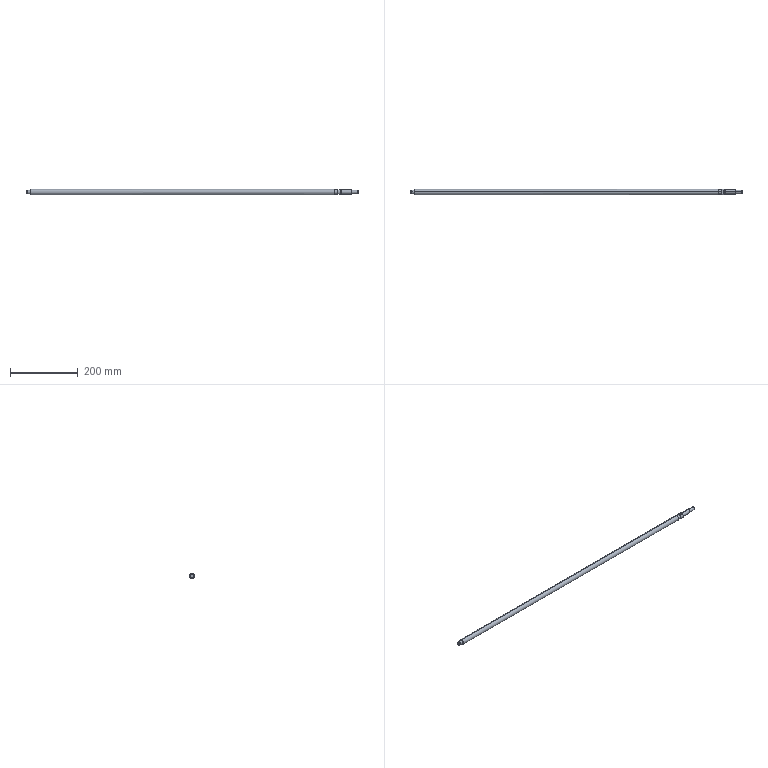Part | STEP file | Ball screw 4R16-16S2-DFSH-920-982-0.05(R)_HIWIN | 1 solid | 44 faces | box 982 x 16 x 16 mm | volume 189994 mm3 | cylinder 17 | plane 17 | cone 10 | commonest cylinder face diameters 10 x6 16 x4 9.6 x2 12 x2 13 x2 3 x1
STEP:
#1=CARTESIAN_POINT('',(-919.5,8.,0.));
#2=VERTEX_POINT('',#1);
#3=CARTESIAN_POINT('',(-919.5,0.,8.));
#4=VERTEX_POINT('',#3);
#5=CARTESIAN_POINT('',(-919.5,0.,0.));
#6=DIRECTION('',(1.,0.,0.));
#7=DIRECTION('',(0.,0.,-1.));
#8=AXIS2_PLACEMENT_3D('',#5,#6,#7);
#9=CIRCLE('',#8,8.);
#10=EDGE_CURVE('',#2,#4,#9,.T.);
#11=ORIENTED_EDGE('',*,*,#10,.T.);
#12=CARTESIAN_POINT('',(-20.,0.,8.));
#13=VERTEX_POINT('',#12);
#14=CARTESIAN_POINT('',(40.657,0.,8.));
#15=DIRECTION('',(1.,0.,0.));
#16=VECTOR('',#15,1000.);
#17=LINE('',#14,#16);
#18=EDGE_CURVE('',#4,#13,#17,.T.);
#19=ORIENTED_EDGE('',*,*,#18,.T.);
#20=CARTESIAN_POINT('',(-20.,0.,-8.));
#21=VERTEX_POINT('',#20);
#22=CARTESIAN_POINT('',(-20.,0.,0.));
#23=DIRECTION('',(-1.,0.,0.));
#24=DIRECTION('',(0.,0.,-1.));
#25=AXIS2_PLACEMENT_3D('',#22,#23,#24);
#26=CIRCLE('',#25,8.);
#27=EDGE_CURVE('',#13,#21,#26,.T.);
#28=ORIENTED_EDGE('',*,*,#27,.T.);
#29=CARTESIAN_POINT('',(-919.5,0.,-8.));
#30=VERTEX_POINT('',#29);
#31=CARTESIAN_POINT('',(40.657,0.,-8.));
#32=DIRECTION('',(1.,0.,0.));
#33=VECTOR('',#32,1000.);
#34=LINE('',#31,#33);
#35=EDGE_CURVE('',#30,#21,#34,.T.);
#36=ORIENTED_EDGE('',*,*,#35,.F.);
#37=CARTESIAN_POINT('',(-919.5,0.,0.));
#38=DIRECTION('',(1.,0.,0.));
#39=DIRECTION('',(0.,0.,-1.));
#40=AXIS2_PLACEMENT_3D('',#37,#38,#39);
#41=CIRCLE('',#40,8.);
#42=EDGE_CURVE('',#30,#2,#41,.T.);
#43=ORIENTED_EDGE('',*,*,#42,.T.);
#44=EDGE_LOOP('',(#11,#19,#28,#36,#43));
#45=FACE_OUTER_BOUND('',#44,.T.);
#46=CARTESIAN_POINT('',(40.657,0.,0.));
#47=DIRECTION('',(1.,0.,0.));
#48=DIRECTION('',(0.,0.,-1.));
#49=AXIS2_PLACEMENT_3D('',#46,#47,#48);
#50=CYLINDRICAL_SURFACE('',#49,8.);
#51=ADVANCED_FACE('',(#45),#50,.T.);
#52=CARTESIAN_POINT('',(-920.,7.5,0.));
#53=VERTEX_POINT('',#52);
#54=CARTESIAN_POINT('',(-920.,-7.5,0.));
#55=VERTEX_POINT('',#54);
#56=CARTESIAN_POINT('',(-920.,0.,0.));
#57=DIRECTION('',(1.,0.,0.));
#58=DIRECTION('',(0.,1.,0.));
#59=AXIS2_PLACEMENT_3D('',#56,#57,#58);
#60=CIRCLE('',#59,7.5);
#61=EDGE_CURVE('',#53,#55,#60,.T.);
#62=ORIENTED_EDGE('',*,*,#61,.T.);
#63=CARTESIAN_POINT('',(-919.5,-8.,0.));
#64=VERTEX_POINT('',#63);
#65=CARTESIAN_POINT('',(-919.5,-8.,0.));
#66=DIRECTION('',(0.7071,-0.7071,0.));
#67=VECTOR('',#66,1000.);
#68=LINE('',#65,#67);
#69=EDGE_CURVE('',#55,#64,#68,.T.);
#70=ORIENTED_EDGE('',*,*,#69,.T.);
#71=CARTESIAN_POINT('',(-919.5,0.,0.));
#72=DIRECTION('',(1.,0.,0.));
#73=DIRECTION('',(0.,0.,-1.));
#74=AXIS2_PLACEMENT_3D('',#71,#72,#73);
#75=CIRCLE('',#74,8.);
#76=EDGE_CURVE('',#4,#64,#75,.T.);
#77=ORIENTED_EDGE('',*,*,#76,.F.);
#78=ORIENTED_EDGE('',*,*,#10,.F.);
#79=CARTESIAN_POINT('',(-919.5,8.,0.));
#80=DIRECTION('',(0.7071,0.7071,0.));
#81=VECTOR('',#80,1000.);
#82=LINE('',#79,#81);
#83=EDGE_CURVE('',#53,#2,#82,.T.);
#84=ORIENTED_EDGE('',*,*,#83,.F.);
#85=EDGE_LOOP('',(#62,#70,#77,#78,#84));
#86=FACE_OUTER_BOUND('',#85,.T.);
#87=CARTESIAN_POINT('',(-919.5,0.,0.));
#88=DIRECTION('',(1.,0.,0.));
#89=DIRECTION('',(0.,1.,0.));
#90=AXIS2_PLACEMENT_3D('',#87,#88,#89);
#91=CONICAL_SURFACE('',#90,8.,0.7854);
#92=ADVANCED_FACE('',(#86),#91,.T.);
#93=CARTESIAN_POINT('',(-20.,0.,6.5));
#94=VERTEX_POINT('',#93);
#95=CARTESIAN_POINT('',(-20.,0.,-6.5));
#96=VERTEX_POINT('',#95);
#97=CARTESIAN_POINT('',(-20.,0.,0.));
#98=DIRECTION('',(-1.,0.,0.));
#99=DIRECTION('',(0.,0.,-1.));
#100=AXIS2_PLACEMENT_3D('',#97,#98,#99);
#101=CIRCLE('',#100,6.5);
#102=EDGE_CURVE('',#94,#96,#101,.T.);
#103=ORIENTED_EDGE('',*,*,#102,.F.);
#104=CARTESIAN_POINT('',(-10.,0.,6.5));
#105=VERTEX_POINT('',#104);
#106=CARTESIAN_POINT('',(-20.,0.,6.5));
#107=DIRECTION('',(1.,0.,0.));
#108=VECTOR('',#107,1000.);
#109=LINE('',#106,#108);
#110=EDGE_CURVE('',#94,#105,#109,.T.);
#111=ORIENTED_EDGE('',*,*,#110,.T.);
#112=CARTESIAN_POINT('',(-10.,0.,-6.5));
#113=VERTEX_POINT('',#112);
#114=CARTESIAN_POINT('',(-10.,0.,0.));
#115=DIRECTION('',(-1.,0.,0.));
#116=DIRECTION('',(0.,0.,-1.));
#117=AXIS2_PLACEMENT_3D('',#114,#115,#116);
#118=CIRCLE('',#117,6.5);
#119=EDGE_CURVE('',#105,#113,#118,.T.);
#120=ORIENTED_EDGE('',*,*,#119,.T.);
#121=CARTESIAN_POINT('',(-20.,0.,-6.5));
#122=DIRECTION('',(1.,0.,0.));
#123=VECTOR('',#122,1000.);
#124=LINE('',#121,#123);
#125=EDGE_CURVE('',#96,#113,#124,.T.);
#126=ORIENTED_EDGE('',*,*,#125,.F.);
#127=EDGE_LOOP('',(#103,#111,#120,#126));
#128=FACE_OUTER_BOUND('',#127,.T.);
#129=CARTESIAN_POINT('',(-20.,0.,0.));
#130=DIRECTION('',(1.,0.,0.));
#131=DIRECTION('',(0.,0.,-1.));
#132=AXIS2_PLACEMENT_3D('',#129,#130,#131);
#133=CYLINDRICAL_SURFACE('',#132,6.5);
#134=ADVANCED_FACE('',(#128),#133,.T.);
#135=CARTESIAN_POINT('',(-928.,0.,-5.));
#136=VERTEX_POINT('',#135);
#137=CARTESIAN_POINT('',(-928.,0.,5.));
#138=VERTEX_POINT('',#137);
#139=CARTESIAN_POINT('',(-928.,0.,0.));
#140=DIRECTION('',(1.,0.,0.));
#141=DIRECTION('',(0.,0.,-1.));
#142=AXIS2_PLACEMENT_3D('',#139,#140,#141);
#143=CIRCLE('',#142,5.);
#144=EDGE_CURVE('',#136,#138,#143,.T.);
#145=ORIENTED_EDGE('',*,*,#144,.T.);
#146=CARTESIAN_POINT('',(-920.,0.,5.));
#147=VERTEX_POINT('',#146);
#148=CARTESIAN_POINT('',(40.657,0.,5.));
#149=DIRECTION('',(1.,0.,0.));
#150=VECTOR('',#149,1000.);
#151=LINE('',#148,#150);
#152=EDGE_CURVE('',#138,#147,#151,.T.);
#153=ORIENTED_EDGE('',*,*,#152,.T.);
#154=CARTESIAN_POINT('',(-920.,0.,-5.));
#155=VERTEX_POINT('',#154);
#156=CARTESIAN_POINT('',(-920.,0.,0.));
#157=DIRECTION('',(1.,0.,0.));
#158=DIRECTION('',(0.,0.,-1.));
#159=AXIS2_PLACEMENT_3D('',#156,#157,#158);
#160=CIRCLE('',#159,5.);
#161=EDGE_CURVE('',#155,#147,#160,.T.);
#162=ORIENTED_EDGE('',*,*,#161,.F.);
#163=CARTESIAN_POINT('',(40.657,0.,-5.));
#164=DIRECTION('',(1.,0.,0.));
#165=VECTOR('',#164,1000.);
#166=LINE('',#163,#165);
#167=EDGE_CURVE('',#136,#155,#166,.T.);
#168=ORIENTED_EDGE('',*,*,#167,.F.);
#169=EDGE_LOOP('',(#145,#153,#162,#168));
#170=FACE_OUTER_BOUND('',#169,.T.);
#171=CARTESIAN_POINT('',(40.657,0.,0.));
#172=DIRECTION('',(1.,0.,0.));
#173=DIRECTION('',(0.,0.,-1.));
#174=AXIS2_PLACEMENT_3D('',#171,#172,#173);
#175=CYLINDRICAL_SURFACE('',#174,5.);
#176=ADVANCED_FACE('',(#170),#175,.T.);
#177=CARTESIAN_POINT('',(-5.,4.664,6.5));
#178=VERTEX_POINT('',#177);
#179=CARTESIAN_POINT('',(-5.,0.,8.));
#180=VERTEX_POINT('',#179);
#181=CARTESIAN_POINT('',(-5.,0.,0.));
#182=DIRECTION('',(1.,0.,0.));
#183=DIRECTION('',(0.,0.,-1.));
#184=AXIS2_PLACEMENT_3D('',#181,#182,#183);
#185=CIRCLE('',#184,8.);
#186=EDGE_CURVE('',#178,#180,#185,.T.);
#187=ORIENTED_EDGE('',*,*,#186,.T.);
#188=CARTESIAN_POINT('',(-0.5,0.,8.));
#189=VERTEX_POINT('',#188);
#190=CARTESIAN_POINT('',(40.657,0.,8.));
#191=DIRECTION('',(1.,0.,0.));
#192=VECTOR('',#191,1000.);
#193=LINE('',#190,#192);
#194=EDGE_CURVE('',#180,#189,#193,.T.);
#195=ORIENTED_EDGE('',*,*,#194,.T.);
#196=CARTESIAN_POINT('',(-0.5,0.,-8.));
#197=VERTEX_POINT('',#196);
#198=CARTESIAN_POINT('',(-0.5,0.,0.));
#199=DIRECTION('',(-1.,0.,0.));
#200=DIRECTION('',(0.,0.,-1.));
#201=AXIS2_PLACEMENT_3D('',#198,#199,#200);
#202=CIRCLE('',#201,8.);
#203=EDGE_CURVE('',#189,#197,#202,.T.);
#204=ORIENTED_EDGE('',*,*,#203,.T.);
#205=CARTESIAN_POINT('',(-5.,0.,-8.));
#206=VERTEX_POINT('',#205);
#207=CARTESIAN_POINT('',(40.657,0.,-8.));
#208=DIRECTION('',(1.,0.,0.));
#209=VECTOR('',#208,1000.);
#210=LINE('',#207,#209);
#211=EDGE_CURVE('',#206,#197,#210,.T.);
#212=ORIENTED_EDGE('',*,*,#211,.F.);
#213=CARTESIAN_POINT('',(-5.,4.664,-6.5));
#214=VERTEX_POINT('',#213);
#215=CARTESIAN_POINT('',(-5.,0.,0.));
#216=DIRECTION('',(1.,0.,0.));
#217=DIRECTION('',(0.,0.,-1.));
#218=AXIS2_PLACEMENT_3D('',#215,#216,#217);
#219=CIRCLE('',#218,8.);
#220=EDGE_CURVE('',#206,#214,#219,.T.);
#221=ORIENTED_EDGE('',*,*,#220,.T.);
#222=CARTESIAN_POINT('',(-10.,4.664,-6.5));
#223=VERTEX_POINT('',#222);
#224=CARTESIAN_POINT('',(-10.,4.664,-6.5));
#225=DIRECTION('',(-1.,0.,0.));
#226=VECTOR('',#225,1000.);
#227=LINE('',#224,#226);
#228=EDGE_CURVE('',#214,#223,#227,.T.);
#229=ORIENTED_EDGE('',*,*,#228,.T.);
#230=CARTESIAN_POINT('',(-10.,4.664,6.5));
#231=VERTEX_POINT('',#230);
#232=CARTESIAN_POINT('',(-10.,0.,0.));
#233=DIRECTION('',(1.,0.,0.));
#234=DIRECTION('',(0.,0.,-1.));
#235=AXIS2_PLACEMENT_3D('',#232,#233,#234);
#236=CIRCLE('',#235,8.);
#237=EDGE_CURVE('',#223,#231,#236,.T.);
#238=ORIENTED_EDGE('',*,*,#237,.T.);
#239=CARTESIAN_POINT('',(-10.,4.664,6.5));
#240=DIRECTION('',(1.,0.,0.));
#241=VECTOR('',#240,1000.);
#242=LINE('',#239,#241);
#243=EDGE_CURVE('',#231,#178,#242,.T.);
#244=ORIENTED_EDGE('',*,*,#243,.T.);
#245=EDGE_LOOP('',(#187,#195,#204,#212,#221,#229,#238,#244));
#246=FACE_OUTER_BOUND('',#245,.T.);
#247=CARTESIAN_POINT('',(40.657,0.,0.));
#248=DIRECTION('',(1.,0.,0.));
#249=DIRECTION('',(0.,0.,-1.));
#250=AXIS2_PLACEMENT_3D('',#247,#248,#249);
#251=CYLINDRICAL_SURFACE('',#250,8.);
#252=ADVANCED_FACE('',(#246),#251,.T.);
#253=CARTESIAN_POINT('',(0.,0.,7.5));
#254=VERTEX_POINT('',#253);
#255=CARTESIAN_POINT('',(0.,0.,-7.5));
#256=VERTEX_POINT('',#255);
#257=CARTESIAN_POINT('',(0.,0.,0.));
#258=DIRECTION('',(-1.,0.,0.));
#259=DIRECTION('',(0.,0.,1.));
#260=AXIS2_PLACEMENT_3D('',#257,#258,#259);
#261=CIRCLE('',#260,7.5);
#262=EDGE_CURVE('',#254,#256,#261,.T.);
#263=ORIENTED_EDGE('',*,*,#262,.T.);
#264=CARTESIAN_POINT('',(-0.5,0.,-8.));
#265=DIRECTION('',(-0.7071,0.,-0.7071));
#266=VECTOR('',#265,1000.);
#267=LINE('',#264,#266);
#268=EDGE_CURVE('',#256,#197,#267,.T.);
#269=ORIENTED_EDGE('',*,*,#268,.T.);
#270=ORIENTED_EDGE('',*,*,#203,.F.);
#271=CARTESIAN_POINT('',(-0.5,0.,8.));
#272=DIRECTION('',(-0.7071,0.,0.7071));
#273=VECTOR('',#272,1000.);
#274=LINE('',#271,#273);
#275=EDGE_CURVE('',#254,#189,#274,.T.);
#276=ORIENTED_EDGE('',*,*,#275,.F.);
#277=EDGE_LOOP('',(#263,#269,#270,#276));
#278=FACE_OUTER_BOUND('',#277,.T.);
#279=CARTESIAN_POINT('',(-0.5,0.,0.));
#280=DIRECTION('',(-1.,0.,0.));
#281=DIRECTION('',(0.,0.,1.));
#282=AXIS2_PLACEMENT_3D('',#279,#280,#281);
#283=CONICAL_SURFACE('',#282,8.,0.7854);
#284=ADVANCED_FACE('',(#278),#283,.T.);
#285=CARTESIAN_POINT('',(-929.15,0.,-4.8));
#286=VERTEX_POINT('',#285);
#287=CARTESIAN_POINT('',(-929.15,0.,4.8));
#288=VERTEX_POINT('',#287);
#289=CARTESIAN_POINT('',(-929.15,0.,0.));
#290=DIRECTION('',(1.,0.,0.));
#291=DIRECTION('',(0.,0.,-1.));
#292=AXIS2_PLACEMENT_3D('',#289,#290,#291);
#293=CIRCLE('',#292,4.8);
#294=EDGE_CURVE('',#286,#288,#293,.T.);
#295=ORIENTED_EDGE('',*,*,#294,.T.);
#296=CARTESIAN_POINT('',(-928.,0.,4.8));
#297=VERTEX_POINT('',#296);
#298=CARTESIAN_POINT('',(40.657,0.,4.8));
#299=DIRECTION('',(1.,0.,0.));
#300=VECTOR('',#299,1000.);
#301=LINE('',#298,#300);
#302=EDGE_CURVE('',#288,#297,#301,.T.);
#303=ORIENTED_EDGE('',*,*,#302,.T.);
#304=CARTESIAN_POINT('',(-928.,0.,-4.8));
#305=VERTEX_POINT('',#304);
#306=CARTESIAN_POINT('',(-928.,0.,0.));
#307=DIRECTION('',(1.,0.,0.));
#308=DIRECTION('',(0.,0.,-1.));
#309=AXIS2_PLACEMENT_3D('',#306,#307,#308);
#310=CIRCLE('',#309,4.8);
#311=EDGE_CURVE('',#305,#297,#310,.T.);
#312=ORIENTED_EDGE('',*,*,#311,.F.);
#313=CARTESIAN_POINT('',(40.657,0.,-4.8));
#314=DIRECTION('',(1.,0.,0.));
#315=VECTOR('',#314,1000.);
#316=LINE('',#313,#315);
#317=EDGE_CURVE('',#286,#305,#316,.T.);
#318=ORIENTED_EDGE('',*,*,#317,.F.);
#319=EDGE_LOOP('',(#295,#303,#312,#318));
#320=FACE_OUTER_BOUND('',#319,.T.);
#321=CARTESIAN_POINT('',(40.657,0.,0.));
#322=DIRECTION('',(1.,0.,0.));
#323=DIRECTION('',(0.,0.,-1.));
#324=AXIS2_PLACEMENT_3D('',#321,#322,#323);
#325=CYLINDRICAL_SURFACE('',#324,4.8);
#326=ADVANCED_FACE('',(#320),#325,.T.);
#327=CARTESIAN_POINT('',(0.,0.,6.));
#328=VERTEX_POINT('',#327);
#329=CARTESIAN_POINT('',(0.,0.,-6.));
#330=VERTEX_POINT('',#329);
#331=CARTESIAN_POINT('',(0.,0.,0.));
#332=DIRECTION('',(-1.,0.,0.));
#333=DIRECTION('',(0.,0.,-1.));
#334=AXIS2_PLACEMENT_3D('',#331,#332,#333);
#335=CIRCLE('',#334,6.);
#336=EDGE_CURVE('',#328,#330,#335,.T.);
#337=ORIENTED_EDGE('',*,*,#336,.F.);
#338=CARTESIAN_POINT('',(29.625,0.,6.));
#339=VERTEX_POINT('',#338);
#340=CARTESIAN_POINT('',(40.657,0.,6.));
#341=DIRECTION('',(1.,0.,0.));
#342=VECTOR('',#341,1000.);
#343=LINE('',#340,#342);
#344=EDGE_CURVE('',#328,#339,#343,.T.);
#345=ORIENTED_EDGE('',*,*,#344,.T.);
#346=CARTESIAN_POINT('',(29.625,0.,-6.));
#347=VERTEX_POINT('',#346);
#348=CARTESIAN_POINT('',(29.625,0.,0.));
#349=DIRECTION('',(-1.,0.,0.));
#350=DIRECTION('',(0.,0.,-1.));
#351=AXIS2_PLACEMENT_3D('',#348,#349,#350);
#352=CIRCLE('',#351,6.);
#353=EDGE_CURVE('',#339,#347,#352,.T.);
#354=ORIENTED_EDGE('',*,*,#353,.T.);
#355=CARTESIAN_POINT('',(40.657,0.,-6.));
#356=DIRECTION('',(1.,0.,0.));
#357=VECTOR('',#356,1000.);
#358=LINE('',#355,#357);
#359=EDGE_CURVE('',#330,#347,#358,.T.);
#360=ORIENTED_EDGE('',*,*,#359,.F.);
#361=EDGE_LOOP('',(#337,#345,#354,#360));
#362=FACE_OUTER_BOUND('',#361,.T.);
#363=CARTESIAN_POINT('',(40.657,0.,0.));
#364=DIRECTION('',(1.,0.,0.));
#365=DIRECTION('',(0.,0.,-1.));
#366=AXIS2_PLACEMENT_3D('',#363,#364,#365);
#367=CYLINDRICAL_SURFACE('',#366,6.);
#368=ADVANCED_FACE('',(#362),#367,.T.);
#369=CARTESIAN_POINT('',(-931.5,0.,-5.));
#370=VERTEX_POINT('',#369);
#371=CARTESIAN_POINT('',(-931.5,0.,5.));
#372=VERTEX_POINT('',#371);
#373=CARTESIAN_POINT('',(-931.5,0.,0.));
#374=DIRECTION('',(1.,0.,0.));
#375=DIRECTION('',(0.,0.,-1.));
#376=AXIS2_PLACEMENT_3D('',#373,#374,#375);
#377=CIRCLE('',#376,5.);
#378=EDGE_CURVE('',#370,#372,#377,.T.);
#379=ORIENTED_EDGE('',*,*,#378,.T.);
#380=CARTESIAN_POINT('',(-929.15,0.,5.));
#381=VERTEX_POINT('',#380);
#382=CARTESIAN_POINT('',(40.657,0.,5.));
#383=DIRECTION('',(1.,0.,0.));
#384=VECTOR('',#383,1000.);
#385=LINE('',#382,#384);
#386=EDGE_CURVE('',#372,#381,#385,.T.);
#387=ORIENTED_EDGE('',*,*,#386,.T.);
#388=CARTESIAN_POINT('',(-929.15,0.,-5.));
#389=VERTEX_POINT('',#388);
#390=CARTESIAN_POINT('',(-929.15,0.,0.));
#391=DIRECTION('',(1.,0.,0.));
#392=DIRECTION('',(0.,0.,-1.));
#393=AXIS2_PLACEMENT_3D('',#390,#391,#392);
#394=CIRCLE('',#393,5.);
#395=EDGE_CURVE('',#389,#381,#394,.T.);
#396=ORIENTED_EDGE('',*,*,#395,.F.);
#397=CARTESIAN_POINT('',(40.657,0.,-5.));
#398=DIRECTION('',(1.,0.,0.));
#399=VECTOR('',#398,1000.);
#400=LINE('',#397,#399);
#401=EDGE_CURVE('',#370,#389,#400,.T.);
#402=ORIENTED_EDGE('',*,*,#401,.F.);
#403=EDGE_LOOP('',(#379,#387,#396,#402));
#404=FACE_OUTER_BOUND('',#403,.T.);
#405=CARTESIAN_POINT('',(40.657,0.,0.));
#406=DIRECTION('',(1.,0.,0.));
#407=DIRECTION('',(0.,0.,-1.));
#408=AXIS2_PLACEMENT_3D('',#405,#406,#407);
#409=CYLINDRICAL_SURFACE('',#408,5.);
#410=ADVANCED_FACE('',(#404),#409,.T.);
#411=CARTESIAN_POINT('',(30.,0.,5.625));
#412=VERTEX_POINT('',#411);
#413=CARTESIAN_POINT('',(30.,0.,-5.625));
#414=VERTEX_POINT('',#413);
#415=CARTESIAN_POINT('',(30.,0.,0.));
#416=DIRECTION('',(-1.,0.,0.));
#417=DIRECTION('',(0.,0.,1.));
#418=AXIS2_PLACEMENT_3D('',#415,#416,#417);
#419=CIRCLE('',#418,5.625);
#420=EDGE_CURVE('',#412,#414,#419,.T.);
#421=ORIENTED_EDGE('',*,*,#420,.T.);
#422=CARTESIAN_POINT('',(29.625,0.,-6.));
#423=DIRECTION('',(-0.7071,0.,-0.7071));
#424=VECTOR('',#423,1000.);
#425=LINE('',#422,#424);
#426=EDGE_CURVE('',#414,#347,#425,.T.);
#427=ORIENTED_EDGE('',*,*,#426,.T.);
#428=ORIENTED_EDGE('',*,*,#353,.F.);
#429=CARTESIAN_POINT('',(29.625,0.,6.));
#430=DIRECTION('',(-0.7071,0.,0.7071));
#431=VECTOR('',#430,1000.);
#432=LINE('',#429,#431);
#433=EDGE_CURVE('',#412,#339,#432,.T.);
#434=ORIENTED_EDGE('',*,*,#433,.F.);
#435=EDGE_LOOP('',(#421,#427,#428,#434));
#436=FACE_OUTER_BOUND('',#435,.T.);
#437=CARTESIAN_POINT('',(29.625,0.,0.));
#438=DIRECTION('',(-1.,0.,0.));
#439=DIRECTION('',(0.,0.,1.));
#440=AXIS2_PLACEMENT_3D('',#437,#438,#439);
#441=CONICAL_SURFACE('',#440,6.,0.7854);
#442=ADVANCED_FACE('',(#436),#441,.T.);
#443=CARTESIAN_POINT('',(-932.,0.,-4.5));
#444=VERTEX_POINT('',#443);
#445=CARTESIAN_POINT('',(-932.,0.,4.5));
#446=VERTEX_POINT('',#445);
#447=CARTESIAN_POINT('',(-932.,0.,0.));
#448=DIRECTION('',(1.,0.,0.));
#449=DIRECTION('',(0.,0.,-1.));
#450=AXIS2_PLACEMENT_3D('',#447,#448,#449);
#451=CIRCLE('',#450,4.5);
#452=EDGE_CURVE('',#444,#446,#451,.T.);
#453=ORIENTED_EDGE('',*,*,#452,.T.);
#454=CARTESIAN_POINT('',(-931.5,0.,5.));
#455=DIRECTION('',(0.7071,0.,0.7071));
#456=VECTOR('',#455,1000.);
#457=LINE('',#454,#456);
#458=EDGE_CURVE('',#446,#372,#457,.T.);
#459=ORIENTED_EDGE('',*,*,#458,.T.);
#460=ORIENTED_EDGE('',*,*,#378,.F.);
#461=CARTESIAN_POINT('',(-931.5,0.,-5.));
#462=DIRECTION('',(0.7071,0.,-0.7071));
#463=VECTOR('',#462,1000.);
#464=LINE('',#461,#463);
#465=EDGE_CURVE('',#444,#370,#464,.T.);
#466=ORIENTED_EDGE('',*,*,#465,.F.);
#467=EDGE_LOOP('',(#453,#459,#460,#466));
#468=FACE_OUTER_BOUND('',#467,.T.);
#469=CARTESIAN_POINT('',(-931.5,0.,0.));
#470=DIRECTION('',(1.,0.,0.));
#471=DIRECTION('',(0.,0.,-1.));
#472=AXIS2_PLACEMENT_3D('',#469,#470,#471);
#473=CONICAL_SURFACE('',#472,5.,0.7854);
#474=ADVANCED_FACE('',(#468),#473,.T.);
#475=CARTESIAN_POINT('',(30.,0.,5.));
#476=VERTEX_POINT('',#475);
#477=CARTESIAN_POINT('',(30.,0.,-5.));
#478=VERTEX_POINT('',#477);
#479=CARTESIAN_POINT('',(30.,0.,0.));
#480=DIRECTION('',(-1.,0.,0.));
#481=DIRECTION('',(0.,0.,-1.));
#482=AXIS2_PLACEMENT_3D('',#479,#480,#481);
#483=CIRCLE('',#482,5.);
#484=EDGE_CURVE('',#476,#478,#483,.T.);
#485=ORIENTED_EDGE('',*,*,#484,.F.);
#486=CARTESIAN_POINT('',(49.5,0.,5.));
#487=VERTEX_POINT('',#486);
#488=CARTESIAN_POINT('',(40.657,0.,5.));
#489=DIRECTION('',(1.,0.,0.));
#490=VECTOR('',#489,1000.);
#491=LINE('',#488,#490);
#492=EDGE_CURVE('',#476,#487,#491,.T.);
#493=ORIENTED_EDGE('',*,*,#492,.T.);
#494=CARTESIAN_POINT('',(49.5,4.77,1.5));
#495=VERTEX_POINT('',#494);
#496=CARTESIAN_POINT('',(49.5,0.,0.));
#497=DIRECTION('',(-1.,0.,0.));
#498=DIRECTION('',(0.,0.,-1.));
#499=AXIS2_PLACEMENT_3D('',#496,#497,#498);
#500=CIRCLE('',#499,5.);
#501=EDGE_CURVE('',#487,#495,#500,.T.);
#502=ORIENTED_EDGE('',*,*,#501,.T.);
#503=CARTESIAN_POINT('',(35.5,4.77,1.5));
#504=VERTEX_POINT('',#503);
#505=CARTESIAN_POINT('',(40.657,4.77,1.5));
#506=DIRECTION('',(-1.,0.,0.));
#507=VECTOR('',#506,1000.);
#508=LINE('',#505,#507);
#509=EDGE_CURVE('',#495,#504,#508,.T.);
#510=ORIENTED_EDGE('',*,*,#509,.T.);
#511=CARTESIAN_POINT('',(35.5,4.77,-1.5));
#512=VERTEX_POINT('',#511);
#513=CARTESIAN_POINT('',(35.5,4.77,1.5));
#514=CARTESIAN_POINT('',(35.4,4.77,1.5));
#515=CARTESIAN_POINT('',(35.302,4.773,1.49));
#516=CARTESIAN_POINT('',(35.11,4.785,1.452));
#517=CARTESIAN_POINT('',(35.014,4.794,1.423));
#518=CARTESIAN_POINT('',(34.833,4.815,1.347));
#519=CARTESIAN_POINT('',(34.747,4.828,1.301));
#520=CARTESIAN_POINT('',(34.585,4.856,1.192));
#521=CARTESIAN_POINT('',(34.508,4.871,1.129));
#522=CARTESIAN_POINT('',(34.302,4.916,0.9233));
#523=CARTESIAN_POINT('',(34.19,4.946,0.7569));
#524=CARTESIAN_POINT('',(34.04,4.988,0.3965));
#525=CARTESIAN_POINT('',(34.,5.,0.1984));
#526=CARTESIAN_POINT('',(34.,5.,-0.09698));
#527=CARTESIAN_POINT('',(34.01,4.997,-0.197));
#528=CARTESIAN_POINT('',(34.048,4.986,-0.3898));
#529=CARTESIAN_POINT('',(34.077,4.977,-0.4837));
#530=CARTESIAN_POINT('',(34.19,4.946,-0.7572));
#531=CARTESIAN_POINT('',(34.301,4.916,-0.9219));
#532=CARTESIAN_POINT('',(34.508,4.871,-1.13));
#533=CARTESIAN_POINT('',(34.583,4.856,-1.191));
#534=CARTESIAN_POINT('',(34.745,4.828,-1.3));
#535=CARTESIAN_POINT('',(34.833,4.815,-1.347));
#536=CARTESIAN_POINT('',(35.104,4.783,-1.46));
#537=CARTESIAN_POINT('',(35.301,4.77,-1.5));
#538=CARTESIAN_POINT('',(35.5,4.77,-1.5));
#539=B_SPLINE_CURVE_WITH_KNOTS('',3,(#513,#514,#515,#516,#517,#518,#519,#520,#521,#522,#523,#524,#525,#526,#527,#528,#529,#530,#531,#532,#533,#534,#535,#536,#537,#538),.UNSPECIFIED.,.F.,.F.,(4,2,2,2,2,2,2,2,2,2,2,2,4),(0.,0.0002947,0.0005894,0.0008841,0.001179,0.001768,0.002358,0.002652,0.002947,0.003536,0.003831,0.004126,0.004715),.UNSPECIFIED.);
#540=EDGE_CURVE('',#504,#512,#539,.T.);
#541=ORIENTED_EDGE('',*,*,#540,.T.);
#542=CARTESIAN_POINT('',(49.5,4.77,-1.5));
#543=VERTEX_POINT('',#542);
#544=CARTESIAN_POINT('',(40.657,4.77,-1.5));
#545=DIRECTION('',(1.,0.,0.));
#546=VECTOR('',#545,1000.);
#547=LINE('',#544,#546);
#548=EDGE_CURVE('',#512,#543,#547,.T.);
#549=ORIENTED_EDGE('',*,*,#548,.T.);
#550=CARTESIAN_POINT('',(49.5,0.,-5.));
#551=VERTEX_POINT('',#550);
#552=CARTESIAN_POINT('',(49.5,0.,0.));
#553=DIRECTION('',(-1.,0.,0.));
#554=DIRECTION('',(0.,0.,-1.));
#555=AXIS2_PLACEMENT_3D('',#552,#553,#554);
#556=CIRCLE('',#555,5.);
#557=EDGE_CURVE('',#543,#551,#556,.T.);
#558=ORIENTED_EDGE('',*,*,#557,.T.);
#559=CARTESIAN_POINT('',(40.657,0.,-5.));
#560=DIRECTION('',(1.,0.,0.));
#561=VECTOR('',#560,1000.);
#562=LINE('',#559,#561);
#563=EDGE_CURVE('',#478,#551,#562,.T.);
#564=ORIENTED_EDGE('',*,*,#563,.F.);
#565=EDGE_LOOP('',(#485,#493,#502,#510,#541,#549,#558,#564));
#566=FACE_OUTER_BOUND('',#565,.T.);
#567=CARTESIAN_POINT('',(40.657,0.,0.));
#568=DIRECTION('',(1.,0.,0.));
#569=DIRECTION('',(0.,0.,-1.));
#570=AXIS2_PLACEMENT_3D('',#567,#568,#569);
#571=CYLINDRICAL_SURFACE('',#570,5.);
#572=ADVANCED_FACE('',(#566),#571,.T.);
#573=CARTESIAN_POINT('',(50.,4.243,-1.5));
#574=VERTEX_POINT('',#573);
#575=CARTESIAN_POINT('',(50.,-4.5,0.));
#576=VERTEX_POINT('',#575);
#577=CARTESIAN_POINT('',(50.,0.,0.));
#578=DIRECTION('',(-1.,0.,0.));
#579=DIRECTION('',(0.,-1.,0.));
#580=AXIS2_PLACEMENT_3D('',#577,#578,#579);
#581=CIRCLE('',#580,4.5);
#582=EDGE_CURVE('',#574,#576,#581,.T.);
#583=ORIENTED_EDGE('',*,*,#582,.T.);
#584=CARTESIAN_POINT('',(49.5,-5.,0.));
#585=VERTEX_POINT('',#584);
#586=CARTESIAN_POINT('',(49.5,-5.,0.));
#587=DIRECTION('',(-0.7071,-0.7071,0.));
#588=VECTOR('',#587,1000.);
#589=LINE('',#586,#588);
#590=EDGE_CURVE('',#576,#585,#589,.T.);
#591=ORIENTED_EDGE('',*,*,#590,.T.);
#592=CARTESIAN_POINT('',(49.5,0.,0.));
#593=DIRECTION('',(-1.,0.,0.));
#594=DIRECTION('',(0.,0.,-1.));
#595=AXIS2_PLACEMENT_3D('',#592,#593,#594);
#596=CIRCLE('',#595,5.);
#597=EDGE_CURVE('',#551,#585,#596,.T.);
#598=ORIENTED_EDGE('',*,*,#597,.F.);
#599=ORIENTED_EDGE('',*,*,#557,.F.);
#600=CARTESIAN_POINT('',(49.5,4.77,-1.5));
#601=CARTESIAN_POINT('',(49.667,4.594,-1.5));
#602=CARTESIAN_POINT('',(49.834,4.419,-1.5));
#603=CARTESIAN_POINT('',(50.,4.243,-1.5));
#604=B_SPLINE_CURVE_WITH_KNOTS('',3,(#600,#601,#602,#603),.UNSPECIFIED.,.F.,.F.,(4,4),(0.,0.0007265),.UNSPECIFIED.);
#605=EDGE_CURVE('',#543,#574,#604,.T.);
#606=ORIENTED_EDGE('',*,*,#605,.T.);
#607=EDGE_LOOP('',(#583,#591,#598,#599,#606));
#608=FACE_OUTER_BOUND('',#607,.T.);
#609=CARTESIAN_POINT('',(49.5,0.,0.));
#610=DIRECTION('',(-1.,0.,0.));
#611=DIRECTION('',(0.,-1.,0.));
#612=AXIS2_PLACEMENT_3D('',#609,#610,#611);
#613=CONICAL_SURFACE('',#612,5.,0.7854);
#614=ADVANCED_FACE('',(#608),#613,.T.);
#615=ORIENTED_EDGE('',*,*,#18,.F.);
#616=ORIENTED_EDGE('',*,*,#76,.T.);
#617=CARTESIAN_POINT('',(-919.5,0.,0.));
#618=DIRECTION('',(1.,0.,0.));
#619=DIRECTION('',(0.,0.,-1.));
#620=AXIS2_PLACEMENT_3D('',#617,#618,#619);
#621=CIRCLE('',#620,8.);
#622=EDGE_CURVE('',#64,#30,#621,.T.);
#623=ORIENTED_EDGE('',*,*,#622,.T.);
#624=ORIENTED_EDGE('',*,*,#35,.T.);
#625=CARTESIAN_POINT('',(-20.,0.,0.));
#626=DIRECTION('',(-1.,0.,0.));
#627=DIRECTION('',(0.,0.,-1.));
#628=AXIS2_PLACEMENT_3D('',#625,#626,#627);
#629=CIRCLE('',#628,8.);
#630=EDGE_CURVE('',#21,#13,#629,.T.);
#631=ORIENTED_EDGE('',*,*,#630,.T.);
#632=EDGE_LOOP('',(#615,#616,#623,#624,#631));
#633=FACE_OUTER_BOUND('',#632,.T.);
#634=CARTESIAN_POINT('',(40.657,0.,0.));
#635=DIRECTION('',(1.,0.,0.));
#636=DIRECTION('',(0.,0.,-1.));
#637=AXIS2_PLACEMENT_3D('',#634,#635,#636);
#638=CYLINDRICAL_SURFACE('',#637,8.);
#639=ADVANCED_FACE('',(#633),#638,.T.);
#640=ORIENTED_EDGE('',*,*,#630,.F.);
#641=ORIENTED_EDGE('',*,*,#27,.F.);
#642=EDGE_LOOP('',(#640,#641));
#643=FACE_OUTER_BOUND('',#642,.T.);
#644=CARTESIAN_POINT('',(-20.,0.,0.));
#645=DIRECTION('',(-1.,0.,0.));
#646=DIRECTION('',(0.,0.,-1.));
#647=AXIS2_PLACEMENT_3D('',#644,#645,#646);
#648=CIRCLE('',#647,6.5);
#649=EDGE_CURVE('',#96,#94,#648,.T.);
#650=ORIENTED_EDGE('',*,*,#649,.T.);
#651=ORIENTED_EDGE('',*,*,#102,.T.);
#652=EDGE_LOOP('',(#650,#651));
#653=FACE_BOUND('',#652,.T.);
#654=CARTESIAN_POINT('',(-20.,0.,0.));
#655=DIRECTION('',(1.,0.,0.));
#656=DIRECTION('',(0.,0.,-1.));
#657=AXIS2_PLACEMENT_3D('',#654,#655,#656);
#658=PLANE('',#657);
#659=ADVANCED_FACE('',(#643,#653),#658,.T.);
#660=ORIENTED_EDGE('',*,*,#69,.F.);
#661=CARTESIAN_POINT('',(-920.,0.,0.));
#662=DIRECTION('',(1.,0.,0.));
#663=DIRECTION('',(0.,1.,0.));
#664=AXIS2_PLACEMENT_3D('',#661,#662,#663);
#665=CIRCLE('',#664,7.5);
#666=EDGE_CURVE('',#55,#53,#665,.T.);
#667=ORIENTED_EDGE('',*,*,#666,.T.);
#668=ORIENTED_EDGE('',*,*,#83,.T.);
#669=ORIENTED_EDGE('',*,*,#42,.F.);
#670=ORIENTED_EDGE('',*,*,#622,.F.);
#671=EDGE_LOOP('',(#660,#667,#668,#669,#670));
#672=FACE_OUTER_BOUND('',#671,.T.);
#673=CARTESIAN_POINT('',(-919.5,0.,0.));
#674=DIRECTION('',(1.,0.,0.));
#675=DIRECTION('',(0.,1.,0.));
#676=AXIS2_PLACEMENT_3D('',#673,#674,#675);
#677=CONICAL_SURFACE('',#676,8.,0.7854);
#678=ADVANCED_FACE('',(#672),#677,.T.);
#679=ORIENTED_EDGE('',*,*,#110,.F.);
#680=ORIENTED_EDGE('',*,*,#649,.F.);
#681=ORIENTED_EDGE('',*,*,#125,.T.);
#682=CARTESIAN_POINT('',(-10.,0.,0.));
#683=DIRECTION('',(-1.,0.,0.));
#684=DIRECTION('',(0.,0.,-1.));
#685=AXIS2_PLACEMENT_3D('',#682,#683,#684);
#686=CIRCLE('',#685,6.5);
#687=EDGE_CURVE('',#113,#105,#686,.T.);
#688=ORIENTED_EDGE('',*,*,#687,.T.);
#689=EDGE_LOOP('',(#679,#680,#681,#688));
#690=FACE_OUTER_BOUND('',#689,.T.);
#691=CARTESIAN_POINT('',(-20.,0.,0.));
#692=DIRECTION('',(1.,0.,0.));
#693=DIRECTION('',(0.,0.,-1.));
#694=AXIS2_PLACEMENT_3D('',#691,#692,#693);
#695=CYLINDRICAL_SURFACE('',#694,6.5);
#696=ADVANCED_FACE('',(#690),#695,.T.);
#697=ORIENTED_EDGE('',*,*,#161,.T.);
#698=CARTESIAN_POINT('',(-920.,0.,0.));
#699=DIRECTION('',(1.,0.,0.));
#700=DIRECTION('',(0.,0.,-1.));
#701=AXIS2_PLACEMENT_3D('',#698,#699,#700);
#702=CIRCLE('',#701,5.);
#703=EDGE_CURVE('',#147,#155,#702,.T.);
#704=ORIENTED_EDGE('',*,*,#703,.T.);
#705=EDGE_LOOP('',(#697,#704));
#706=FACE_BOUND('',#705,.T.);
#707=ORIENTED_EDGE('',*,*,#61,.F.);
#708=ORIENTED_EDGE('',*,*,#666,.F.);
#709=EDGE_LOOP('',(#707,#708));
#710=FACE_OUTER_BOUND('',#709,.T.);
#711=CARTESIAN_POINT('',(-920.,8.,0.));
#712=DIRECTION('',(-1.,0.,0.));
#713=DIRECTION('',(0.,0.,1.));
#714=AXIS2_PLACEMENT_3D('',#711,#712,#713);
#715=PLANE('',#714);
#716=ADVANCED_FACE('',(#706,#710),#715,.T.);
#717=CARTESIAN_POINT('',(-10.,-4.664,6.5));
#718=VERTEX_POINT('',#717);
#719=CARTESIAN_POINT('',(-10.,0.,6.5));
#720=DIRECTION('',(0.,-1.,0.));
#721=VECTOR('',#720,1000.);
#722=LINE('',#719,#721);
#723=EDGE_CURVE('',#105,#718,#722,.T.);
#724=ORIENTED_EDGE('',*,*,#723,.F.);
#725=ORIENTED_EDGE('',*,*,#687,.F.);
#726=CARTESIAN_POINT('',(-10.,-4.664,-6.5));
#727=VERTEX_POINT('',#726);
#728=CARTESIAN_POINT('',(-10.,0.,-6.5));
#729=DIRECTION('',(0.,1.,0.));
#730=VECTOR('',#729,1000.);
#731=LINE('',#728,#730);
#732=EDGE_CURVE('',#727,#113,#731,.T.);
#733=ORIENTED_EDGE('',*,*,#732,.F.);
#734=CARTESIAN_POINT('',(-10.,0.,0.));
#735=DIRECTION('',(1.,0.,0.));
#736=DIRECTION('',(0.,0.,-1.));
#737=AXIS2_PLACEMENT_3D('',#734,#735,#736);
#738=CIRCLE('',#737,8.);
#739=EDGE_CURVE('',#718,#727,#738,.T.);
#740=ORIENTED_EDGE('',*,*,#739,.F.);
#741=EDGE_LOOP('',(#724,#725,#733,#740));
#742=FACE_OUTER_BOUND('',#741,.T.);
#743=CARTESIAN_POINT('',(-10.,0.,0.));
#744=DIRECTION('',(1.,0.,0.));
#745=DIRECTION('',(0.,0.,-1.));
#746=AXIS2_PLACEMENT_3D('',#743,#744,#745);
#747=PLANE('',#746);
#748=ADVANCED_FACE('',(#742),#747,.F.);
#749=CARTESIAN_POINT('',(-10.,0.,6.5));
#750=DIRECTION('',(0.,-1.,0.));
#751=VECTOR('',#750,1000.);
#752=LINE('',#749,#751);
#753=EDGE_CURVE('',#231,#105,#752,.T.);
#754=ORIENTED_EDGE('',*,*,#753,.F.);
#755=ORIENTED_EDGE('',*,*,#237,.F.);
#756=CARTESIAN_POINT('',(-10.,0.,-6.5));
#757=DIRECTION('',(0.,1.,0.));
#758=VECTOR('',#757,1000.);
#759=LINE('',#756,#758);
#760=EDGE_CURVE('',#113,#223,#759,.T.);
#761=ORIENTED_EDGE('',*,*,#760,.F.);
#762=ORIENTED_EDGE('',*,*,#119,.F.);
#763=EDGE_LOOP('',(#754,#755,#761,#762));
#764=FACE_OUTER_BOUND('',#763,.T.);
#765=CARTESIAN_POINT('',(-10.,0.,0.));
#766=DIRECTION('',(1.,0.,0.));
#767=DIRECTION('',(0.,0.,-1.));
#768=AXIS2_PLACEMENT_3D('',#765,#766,#767);
#769=PLANE('',#768);
#770=ADVANCED_FACE('',(#764),#769,.F.);
#771=ORIENTED_EDGE('',*,*,#152,.F.);
#772=CARTESIAN_POINT('',(-928.,0.,0.));
#773=DIRECTION('',(1.,0.,0.));
#774=DIRECTION('',(0.,0.,-1.));
#775=AXIS2_PLACEMENT_3D('',#772,#773,#774);
#776=CIRCLE('',#775,5.);
#777=EDGE_CURVE('',#138,#136,#776,.T.);
#778=ORIENTED_EDGE('',*,*,#777,.T.);
#779=ORIENTED_EDGE('',*,*,#167,.T.);
#780=ORIENTED_EDGE('',*,*,#703,.F.);
#781=EDGE_LOOP('',(#771,#778,#779,#780));
#782=FACE_OUTER_BOUND('',#781,.T.);
#783=CARTESIAN_POINT('',(40.657,0.,0.));
#784=DIRECTION('',(1.,0.,0.));
#785=DIRECTION('',(0.,0.,-1.));
#786=AXIS2_PLACEMENT_3D('',#783,#784,#785);
#787=CYLINDRICAL_SURFACE('',#786,5.);
#788=ADVANCED_FACE('',(#782),#787,.T.);
#789=ORIENTED_EDGE('',*,*,#194,.F.);
#790=CARTESIAN_POINT('',(-5.,-4.664,6.5));
#791=VERTEX_POINT('',#790);
#792=CARTESIAN_POINT('',(-5.,0.,0.));
#793=DIRECTION('',(1.,0.,0.));
#794=DIRECTION('',(0.,0.,-1.));
#795=AXIS2_PLACEMENT_3D('',#792,#793,#794);
#796=CIRCLE('',#795,8.);
#797=EDGE_CURVE('',#180,#791,#796,.T.);
#798=ORIENTED_EDGE('',*,*,#797,.T.);
#799=CARTESIAN_POINT('',(40.657,-4.664,6.5));
#800=DIRECTION('',(-1.,0.,0.));
#801=VECTOR('',#800,1000.);
#802=LINE('',#799,#801);
#803=EDGE_CURVE('',#791,#718,#802,.T.);
#804=ORIENTED_EDGE('',*,*,#803,.T.);
#805=ORIENTED_EDGE('',*,*,#739,.T.);
#806=CARTESIAN_POINT('',(-5.,-4.664,-6.5));
#807=VERTEX_POINT('',#806);
#808=CARTESIAN_POINT('',(40.657,-4.664,-6.5));
#809=DIRECTION('',(1.,0.,0.));
#810=VECTOR('',#809,1000.);
#811=LINE('',#808,#810);
#812=EDGE_CURVE('',#727,#807,#811,.T.);
#813=ORIENTED_EDGE('',*,*,#812,.T.);
#814=CARTESIAN_POINT('',(-5.,0.,0.));
#815=DIRECTION('',(1.,0.,0.));
#816=DIRECTION('',(0.,0.,-1.));
#817=AXIS2_PLACEMENT_3D('',#814,#815,#816);
#818=CIRCLE('',#817,8.);
#819=EDGE_CURVE('',#807,#206,#818,.T.);
#820=ORIENTED_EDGE('',*,*,#819,.T.);
#821=ORIENTED_EDGE('',*,*,#211,.T.);
#822=CARTESIAN_POINT('',(-0.5,0.,0.));
#823=DIRECTION('',(-1.,0.,0.));
#824=DIRECTION('',(0.,0.,-1.));
#825=AXIS2_PLACEMENT_3D('',#822,#823,#824);
#826=CIRCLE('',#825,8.);
#827=EDGE_CURVE('',#197,#189,#826,.T.);
#828=ORIENTED_EDGE('',*,*,#827,.T.);
#829=EDGE_LOOP('',(#789,#798,#804,#805,#813,#820,#821,#828));
#830=FACE_OUTER_BOUND('',#829,.T.);
#831=CARTESIAN_POINT('',(40.657,0.,0.));
#832=DIRECTION('',(1.,0.,0.));
#833=DIRECTION('',(0.,0.,-1.));
#834=AXIS2_PLACEMENT_3D('',#831,#832,#833);
#835=CYLINDRICAL_SURFACE('',#834,8.);
#836=ADVANCED_FACE('',(#830),#835,.T.);
#837=ORIENTED_EDGE('',*,*,#753,.T.);
#838=ORIENTED_EDGE('',*,*,#723,.T.);
#839=ORIENTED_EDGE('',*,*,#803,.F.);
#840=CARTESIAN_POINT('',(-5.,-8.,6.5));
#841=DIRECTION('',(0.,-1.,0.));
#842=VECTOR('',#841,1000.);
#843=LINE('',#840,#842);
#844=EDGE_CURVE('',#178,#791,#843,.T.);
#845=ORIENTED_EDGE('',*,*,#844,.F.);
#846=ORIENTED_EDGE('',*,*,#243,.F.);
#847=EDGE_LOOP('',(#837,#838,#839,#845,#846));
#848=FACE_OUTER_BOUND('',#847,.T.);
#849=CARTESIAN_POINT('',(-10.,-8.,6.5));
#850=DIRECTION('',(0.,0.,-1.));
#851=DIRECTION('',(-1.,0.,0.));
#852=AXIS2_PLACEMENT_3D('',#849,#850,#851);
#853=PLANE('',#852);
#854=ADVANCED_FACE('',(#848),#853,.F.);
#855=ORIENTED_EDGE('',*,*,#732,.T.);
#856=ORIENTED_EDGE('',*,*,#760,.T.);
#857=ORIENTED_EDGE('',*,*,#228,.F.);
#858=CARTESIAN_POINT('',(-5.,-8.,-6.5));
#859=DIRECTION('',(0.,1.,0.));
#860=VECTOR('',#859,1000.);
#861=LINE('',#858,#860);
#862=EDGE_CURVE('',#807,#214,#861,.T.);
#863=ORIENTED_EDGE('',*,*,#862,.F.);
#864=ORIENTED_EDGE('',*,*,#812,.F.);
#865=EDGE_LOOP('',(#855,#856,#857,#863,#864));
#866=FACE_OUTER_BOUND('',#865,.T.);
#867=CARTESIAN_POINT('',(-10.,-8.,-6.5));
#868=DIRECTION('',(0.,0.,1.));
#869=DIRECTION('',(1.,0.,0.));
#870=AXIS2_PLACEMENT_3D('',#867,#868,#869);
#871=PLANE('',#870);
#872=ADVANCED_FACE('',(#866),#871,.F.);
#873=ORIENTED_EDGE('',*,*,#144,.F.);
#874=ORIENTED_EDGE('',*,*,#777,.F.);
#875=EDGE_LOOP('',(#873,#874));
#876=FACE_OUTER_BOUND('',#875,.T.);
#877=ORIENTED_EDGE('',*,*,#311,.T.);
#878=CARTESIAN_POINT('',(-928.,0.,0.));
#879=DIRECTION('',(1.,0.,0.));
#880=DIRECTION('',(0.,0.,-1.));
#881=AXIS2_PLACEMENT_3D('',#878,#879,#880);
#882=CIRCLE('',#881,4.8);
#883=EDGE_CURVE('',#297,#305,#882,.T.);
#884=ORIENTED_EDGE('',*,*,#883,.T.);
#885=EDGE_LOOP('',(#877,#884));
#886=FACE_BOUND('',#885,.T.);
#887=CARTESIAN_POINT('',(-928.,5.,0.));
#888=DIRECTION('',(-1.,0.,0.));
#889=DIRECTION('',(0.,0.,1.));
#890=AXIS2_PLACEMENT_3D('',#887,#888,#889);
#891=PLANE('',#890);
#892=ADVANCED_FACE('',(#876,#886),#891,.T.);
#893=ORIENTED_EDGE('',*,*,#268,.F.);
#894=CARTESIAN_POINT('',(0.,0.,0.));
#895=DIRECTION('',(-1.,0.,0.));
#896=DIRECTION('',(0.,0.,1.));
#897=AXIS2_PLACEMENT_3D('',#894,#895,#896);
#898=CIRCLE('',#897,7.5);
#899=EDGE_CURVE('',#256,#254,#898,.T.);
#900=ORIENTED_EDGE('',*,*,#899,.T.);
#901=ORIENTED_EDGE('',*,*,#275,.T.);
#902=ORIENTED_EDGE('',*,*,#827,.F.);
#903=EDGE_LOOP('',(#893,#900,#901,#902));
#904=FACE_OUTER_BOUND('',#903,.T.);
#905=CARTESIAN_POINT('',(-0.5,0.,0.));
#906=DIRECTION('',(-1.,0.,0.));
#907=DIRECTION('',(0.,0.,1.));
#908=AXIS2_PLACEMENT_3D('',#905,#906,#907);
#909=CONICAL_SURFACE('',#908,8.,0.7854);
#910=ADVANCED_FACE('',(#904),#909,.T.);
#911=ORIENTED_EDGE('',*,*,#819,.F.);
#912=ORIENTED_EDGE('',*,*,#862,.T.);
#913=ORIENTED_EDGE('',*,*,#220,.F.);
#914=EDGE_LOOP('',(#911,#912,#913));
#915=FACE_OUTER_BOUND('',#914,.T.);
#916=CARTESIAN_POINT('',(-5.,-8.,-8.));
#917=DIRECTION('',(1.,0.,0.));
#918=DIRECTION('',(0.,0.,-1.));
#919=AXIS2_PLACEMENT_3D('',#916,#917,#918);
#920=PLANE('',#919);
#921=ADVANCED_FACE('',(#915),#920,.F.);
#922=ORIENTED_EDGE('',*,*,#186,.F.);
#923=ORIENTED_EDGE('',*,*,#844,.T.);
#924=ORIENTED_EDGE('',*,*,#797,.F.);
#925=EDGE_LOOP('',(#922,#923,#924));
#926=FACE_OUTER_BOUND('',#925,.T.);
#927=CARTESIAN_POINT('',(-5.,-8.,8.));
#928=DIRECTION('',(1.,0.,0.));
#929=DIRECTION('',(0.,0.,-1.));
#930=AXIS2_PLACEMENT_3D('',#927,#928,#929);
#931=PLANE('',#930);
#932=ADVANCED_FACE('',(#926),#931,.F.);
#933=ORIENTED_EDGE('',*,*,#302,.F.);
#934=CARTESIAN_POINT('',(-929.15,0.,0.));
#935=DIRECTION('',(1.,0.,0.));
#936=DIRECTION('',(0.,0.,-1.));
#937=AXIS2_PLACEMENT_3D('',#934,#935,#936);
#938=CIRCLE('',#937,4.8);
#939=EDGE_CURVE('',#288,#286,#938,.T.);
#940=ORIENTED_EDGE('',*,*,#939,.T.);
#941=ORIENTED_EDGE('',*,*,#317,.T.);
#942=ORIENTED_EDGE('',*,*,#883,.F.);
#943=EDGE_LOOP('',(#933,#940,#941,#942));
#944=FACE_OUTER_BOUND('',#943,.T.);
#945=CARTESIAN_POINT('',(40.657,0.,0.));
#946=DIRECTION('',(1.,0.,0.));
#947=DIRECTION('',(0.,0.,-1.));
#948=AXIS2_PLACEMENT_3D('',#945,#946,#947);
#949=CYLINDRICAL_SURFACE('',#948,4.8);
#950=ADVANCED_FACE('',(#944),#949,.T.);
#951=CARTESIAN_POINT('',(0.,0.,0.));
#952=DIRECTION('',(-1.,0.,0.));
#953=DIRECTION('',(0.,0.,-1.));
#954=AXIS2_PLACEMENT_3D('',#951,#952,#953);
#955=CIRCLE('',#954,6.);
#956=EDGE_CURVE('',#330,#328,#955,.T.);
#957=ORIENTED_EDGE('',*,*,#956,.T.);
#958=ORIENTED_EDGE('',*,*,#336,.T.);
#959=EDGE_LOOP('',(#957,#958));
#960=FACE_BOUND('',#959,.T.);
#961=ORIENTED_EDGE('',*,*,#262,.F.);
#962=ORIENTED_EDGE('',*,*,#899,.F.);
#963=EDGE_LOOP('',(#961,#962));
#964=FACE_OUTER_BOUND('',#963,.T.);
#965=CARTESIAN_POINT('',(0.,6.,0.));
#966=DIRECTION('',(1.,0.,0.));
#967=DIRECTION('',(0.,0.,-1.));
#968=AXIS2_PLACEMENT_3D('',#965,#966,#967);
#969=PLANE('',#968);
#970=ADVANCED_FACE('',(#960,#964),#969,.T.);
#971=ORIENTED_EDGE('',*,*,#294,.F.);
#972=ORIENTED_EDGE('',*,*,#939,.F.);
#973=EDGE_LOOP('',(#971,#972));
#974=FACE_BOUND('',#973,.T.);
#975=ORIENTED_EDGE('',*,*,#395,.T.);
#976=CARTESIAN_POINT('',(-929.15,0.,0.));
#977=DIRECTION('',(1.,0.,0.));
#978=DIRECTION('',(0.,0.,-1.));
#979=AXIS2_PLACEMENT_3D('',#976,#977,#978);
#980=CIRCLE('',#979,5.);
#981=EDGE_CURVE('',#381,#389,#980,.T.);
#982=ORIENTED_EDGE('',*,*,#981,.T.);
#983=EDGE_LOOP('',(#975,#982));
#984=FACE_OUTER_BOUND('',#983,.T.);
#985=CARTESIAN_POINT('',(-929.15,4.8,0.));
#986=DIRECTION('',(1.,0.,0.));
#987=DIRECTION('',(0.,0.,-1.));
#988=AXIS2_PLACEMENT_3D('',#985,#986,#987);
#989=PLANE('',#988);
#990=ADVANCED_FACE('',(#974,#984),#989,.T.);
#991=ORIENTED_EDGE('',*,*,#344,.F.);
#992=ORIENTED_EDGE('',*,*,#956,.F.);
#993=ORIENTED_EDGE('',*,*,#359,.T.);
#994=CARTESIAN_POINT('',(29.625,0.,0.));
#995=DIRECTION('',(-1.,0.,0.));
#996=DIRECTION('',(0.,0.,-1.));
#997=AXIS2_PLACEMENT_3D('',#994,#995,#996);
#998=CIRCLE('',#997,6.);
#999=EDGE_CURVE('',#347,#339,#998,.T.);
#1000=ORIENTED_EDGE('',*,*,#999,.T.);
#1001=EDGE_LOOP('',(#991,#992,#993,#1000));
#1002=FACE_OUTER_BOUND('',#1001,.T.);
#1003=CARTESIAN_POINT('',(40.657,0.,0.));
#1004=DIRECTION('',(1.,0.,0.));
#1005=DIRECTION('',(0.,0.,-1.));
#1006=AXIS2_PLACEMENT_3D('',#1003,#1004,#1005);
#1007=CYLINDRICAL_SURFACE('',#1006,6.);
#1008=ADVANCED_FACE('',(#1002),#1007,.T.);
#1009=ORIENTED_EDGE('',*,*,#386,.F.);
#1010=CARTESIAN_POINT('',(-931.5,0.,0.));
#1011=DIRECTION('',(1.,0.,0.));
#1012=DIRECTION('',(0.,0.,-1.));
#1013=AXIS2_PLACEMENT_3D('',#1010,#1011,#1012);
#1014=CIRCLE('',#1013,5.);
#1015=EDGE_CURVE('',#372,#370,#1014,.T.);
#1016=ORIENTED_EDGE('',*,*,#1015,.T.);
#1017=ORIENTED_EDGE('',*,*,#401,.T.);
#1018=ORIENTED_EDGE('',*,*,#981,.F.);
#1019=EDGE_LOOP('',(#1009,#1016,#1017,#1018));
#1020=FACE_OUTER_BOUND('',#1019,.T.);
#1021=CARTESIAN_POINT('',(40.657,0.,0.));
#1022=DIRECTION('',(1.,0.,0.));
#1023=DIRECTION('',(0.,0.,-1.));
#1024=AXIS2_PLACEMENT_3D('',#1021,#1022,#1023);
#1025=CYLINDRICAL_SURFACE('',#1024,5.);
#1026=ADVANCED_FACE('',(#1020),#1025,.T.);
#1027=ORIENTED_EDGE('',*,*,#426,.F.);
#1028=CARTESIAN_POINT('',(30.,0.,0.));
#1029=DIRECTION('',(-1.,0.,0.));
#1030=DIRECTION('',(0.,0.,1.));
#1031=AXIS2_PLACEMENT_3D('',#1028,#1029,#1030);
#1032=CIRCLE('',#1031,5.625);
#1033=EDGE_CURVE('',#414,#412,#1032,.T.);
#1034=ORIENTED_EDGE('',*,*,#1033,.T.);
#1035=ORIENTED_EDGE('',*,*,#433,.T.);
#1036=ORIENTED_EDGE('',*,*,#999,.F.);
#1037=EDGE_LOOP('',(#1027,#1034,#1035,#1036));
#1038=FACE_OUTER_BOUND('',#1037,.T.);
#1039=CARTESIAN_POINT('',(29.625,0.,0.));
#1040=DIRECTION('',(-1.,0.,0.));
#1041=DIRECTION('',(0.,0.,1.));
#1042=AXIS2_PLACEMENT_3D('',#1039,#1040,#1041);
#1043=CONICAL_SURFACE('',#1042,6.,0.7854);
#1044=ADVANCED_FACE('',(#1038),#1043,.T.);
#1045=ORIENTED_EDGE('',*,*,#458,.F.);
#1046=CARTESIAN_POINT('',(-932.,0.,0.));
#1047=DIRECTION('',(1.,0.,0.));
#1048=DIRECTION('',(0.,0.,-1.));
#1049=AXIS2_PLACEMENT_3D('',#1046,#1047,#1048);
#1050=CIRCLE('',#1049,4.5);
#1051=EDGE_CURVE('',#446,#444,#1050,.T.);
#1052=ORIENTED_EDGE('',*,*,#1051,.T.);
#1053=ORIENTED_EDGE('',*,*,#465,.T.);
#1054=ORIENTED_EDGE('',*,*,#1015,.F.);
#1055=EDGE_LOOP('',(#1045,#1052,#1053,#1054));
#1056=FACE_OUTER_BOUND('',#1055,.T.);
#1057=CARTESIAN_POINT('',(-931.5,0.,0.));
#1058=DIRECTION('',(1.,0.,0.));
#1059=DIRECTION('',(0.,0.,-1.));
#1060=AXIS2_PLACEMENT_3D('',#1057,#1058,#1059);
#1061=CONICAL_SURFACE('',#1060,5.,0.7854);
#1062=ADVANCED_FACE('',(#1056),#1061,.T.);
#1063=CARTESIAN_POINT('',(30.,0.,0.));
#1064=DIRECTION('',(-1.,0.,0.));
#1065=DIRECTION('',(0.,0.,-1.));
#1066=AXIS2_PLACEMENT_3D('',#1063,#1064,#1065);
#1067=CIRCLE('',#1066,5.);
#1068=EDGE_CURVE('',#478,#476,#1067,.T.);
#1069=ORIENTED_EDGE('',*,*,#1068,.T.);
#1070=ORIENTED_EDGE('',*,*,#484,.T.);
#1071=EDGE_LOOP('',(#1069,#1070));
#1072=FACE_BOUND('',#1071,.T.);
#1073=ORIENTED_EDGE('',*,*,#420,.F.);
#1074=ORIENTED_EDGE('',*,*,#1033,.F.);
#1075=EDGE_LOOP('',(#1073,#1074));
#1076=FACE_OUTER_BOUND('',#1075,.T.);
#1077=CARTESIAN_POINT('',(30.,5.,0.));
#1078=DIRECTION('',(1.,0.,0.));
#1079=DIRECTION('',(0.,0.,-1.));
#1080=AXIS2_PLACEMENT_3D('',#1077,#1078,#1079);
#1081=PLANE('',#1080);
#1082=ADVANCED_FACE('',(#1072,#1076),#1081,.T.);
#1083=ORIENTED_EDGE('',*,*,#452,.F.);
#1084=ORIENTED_EDGE('',*,*,#1051,.F.);
#1085=EDGE_LOOP('',(#1083,#1084));
#1086=FACE_OUTER_BOUND('',#1085,.T.);
#1087=CARTESIAN_POINT('',(-932.,5.,0.));
#1088=DIRECTION('',(-1.,0.,0.));
#1089=DIRECTION('',(0.,0.,1.));
#1090=AXIS2_PLACEMENT_3D('',#1087,#1088,#1089);
#1091=PLANE('',#1090);
#1092=ADVANCED_FACE('',(#1086),#1091,.T.);
#1093=ORIENTED_EDGE('',*,*,#492,.F.);
#1094=ORIENTED_EDGE('',*,*,#1068,.F.);
#1095=ORIENTED_EDGE('',*,*,#563,.T.);
#1096=ORIENTED_EDGE('',*,*,#597,.T.);
#1097=CARTESIAN_POINT('',(49.5,0.,0.));
#1098=DIRECTION('',(-1.,0.,0.));
#1099=DIRECTION('',(0.,0.,-1.));
#1100=AXIS2_PLACEMENT_3D('',#1097,#1098,#1099);
#1101=CIRCLE('',#1100,5.);
#1102=EDGE_CURVE('',#585,#487,#1101,.T.);
#1103=ORIENTED_EDGE('',*,*,#1102,.T.);
#1104=EDGE_LOOP('',(#1093,#1094,#1095,#1096,#1103));
#1105=FACE_OUTER_BOUND('',#1104,.T.);
#1106=CARTESIAN_POINT('',(40.657,0.,0.));
#1107=DIRECTION('',(1.,0.,0.));
#1108=DIRECTION('',(0.,0.,-1.));
#1109=AXIS2_PLACEMENT_3D('',#1106,#1107,#1108);
#1110=CYLINDRICAL_SURFACE('',#1109,5.);
#1111=ADVANCED_FACE('',(#1105),#1110,.T.);
#1112=ORIENTED_EDGE('',*,*,#590,.F.);
#1113=CARTESIAN_POINT('',(50.,4.243,1.5));
#1114=VERTEX_POINT('',#1113);
#1115=CARTESIAN_POINT('',(50.,0.,0.));
#1116=DIRECTION('',(-1.,0.,0.));
#1117=DIRECTION('',(0.,-1.,0.));
#1118=AXIS2_PLACEMENT_3D('',#1115,#1116,#1117);
#1119=CIRCLE('',#1118,4.5);
#1120=EDGE_CURVE('',#576,#1114,#1119,.T.);
#1121=ORIENTED_EDGE('',*,*,#1120,.T.);
#1122=CARTESIAN_POINT('',(49.5,4.77,1.5));
#1123=CARTESIAN_POINT('',(49.667,4.594,1.5));
#1124=CARTESIAN_POINT('',(49.834,4.419,1.5));
#1125=CARTESIAN_POINT('',(50.,4.243,1.5));
#1126=B_SPLINE_CURVE_WITH_KNOTS('',3,(#1122,#1123,#1124,#1125),.UNSPECIFIED.,.F.,.F.,(4,4),(0.,0.0007265),.UNSPECIFIED.);
#1127=EDGE_CURVE('',#495,#1114,#1126,.T.);
#1128=ORIENTED_EDGE('',*,*,#1127,.F.);
#1129=ORIENTED_EDGE('',*,*,#501,.F.);
#1130=ORIENTED_EDGE('',*,*,#1102,.F.);
#1131=EDGE_LOOP('',(#1112,#1121,#1128,#1129,#1130));
#1132=FACE_OUTER_BOUND('',#1131,.T.);
#1133=CARTESIAN_POINT('',(49.5,0.,0.));
#1134=DIRECTION('',(-1.,0.,0.));
#1135=DIRECTION('',(0.,-1.,0.));
#1136=AXIS2_PLACEMENT_3D('',#1133,#1134,#1135);
#1137=CONICAL_SURFACE('',#1136,5.,0.7854);
#1138=ADVANCED_FACE('',(#1132),#1137,.T.);
#1139=ORIENTED_EDGE('',*,*,#605,.F.);
#1140=ORIENTED_EDGE('',*,*,#548,.F.);
#1141=CARTESIAN_POINT('',(35.5,3.2,-1.5));
#1142=VERTEX_POINT('',#1141);
#1143=CARTESIAN_POINT('',(35.5,13.2,-1.5));
#1144=DIRECTION('',(0.,-1.,0.));
#1145=VECTOR('',#1144,1000.);
#1146=LINE('',#1143,#1145);
#1147=EDGE_CURVE('',#512,#1142,#1146,.T.);
#1148=ORIENTED_EDGE('',*,*,#1147,.T.);
#1149=CARTESIAN_POINT('',(50.,3.2,-1.5));
#1150=VERTEX_POINT('',#1149);
#1151=CARTESIAN_POINT('',(50.,3.2,-1.5));
#1152=DIRECTION('',(1.,0.,0.));
#1153=VECTOR('',#1152,1000.);
#1154=LINE('',#1151,#1153);
#1155=EDGE_CURVE('',#1142,#1150,#1154,.T.);
#1156=ORIENTED_EDGE('',*,*,#1155,.T.);
#1157=CARTESIAN_POINT('',(50.,13.2,-1.5));
#1158=DIRECTION('',(0.,1.,0.));
#1159=VECTOR('',#1158,1000.);
#1160=LINE('',#1157,#1159);
#1161=EDGE_CURVE('',#1150,#574,#1160,.T.);
#1162=ORIENTED_EDGE('',*,*,#1161,.T.);
#1163=EDGE_LOOP('',(#1139,#1140,#1148,#1156,#1162));
#1164=FACE_OUTER_BOUND('',#1163,.T.);
#1165=CARTESIAN_POINT('',(50.,13.2,-1.5));
#1166=DIRECTION('',(0.,0.,1.));
#1167=DIRECTION('',(1.,0.,0.));
#1168=AXIS2_PLACEMENT_3D('',#1165,#1166,#1167);
#1169=PLANE('',#1168);
#1170=ADVANCED_FACE('',(#1164),#1169,.T.);
#1171=CARTESIAN_POINT('',(35.5,3.2,1.5));
#1172=VERTEX_POINT('',#1171);
#1173=CARTESIAN_POINT('',(35.5,3.2,0.));
#1174=DIRECTION('',(0.,1.,0.));
#1175=DIRECTION('',(0.,0.,-1.));
#1176=AXIS2_PLACEMENT_3D('',#1173,#1174,#1175);
#1177=CIRCLE('',#1176,1.5);
#1178=EDGE_CURVE('',#1142,#1172,#1177,.T.);
#1179=ORIENTED_EDGE('',*,*,#1178,.F.);
#1180=ORIENTED_EDGE('',*,*,#1147,.F.);
#1181=ORIENTED_EDGE('',*,*,#540,.F.);
#1182=CARTESIAN_POINT('',(35.5,13.2,1.5));
#1183=DIRECTION('',(0.,1.,0.));
#1184=VECTOR('',#1183,1000.);
#1185=LINE('',#1182,#1184);
#1186=EDGE_CURVE('',#1172,#504,#1185,.T.);
#1187=ORIENTED_EDGE('',*,*,#1186,.F.);
#1188=EDGE_LOOP('',(#1179,#1180,#1181,#1187));
#1189=FACE_OUTER_BOUND('',#1188,.T.);
#1190=CARTESIAN_POINT('',(35.5,13.2,0.));
#1191=DIRECTION('',(0.,-1.,0.));
#1192=DIRECTION('',(0.,0.,-1.));
#1193=AXIS2_PLACEMENT_3D('',#1190,#1191,#1192);
#1194=CYLINDRICAL_SURFACE('',#1193,1.5);
#1195=ADVANCED_FACE('',(#1189),#1194,.F.);
#1196=ORIENTED_EDGE('',*,*,#1186,.T.);
#1197=ORIENTED_EDGE('',*,*,#509,.F.);
#1198=ORIENTED_EDGE('',*,*,#1127,.T.);
#1199=CARTESIAN_POINT('',(50.,3.2,1.5));
#1200=VERTEX_POINT('',#1199);
#1201=CARTESIAN_POINT('',(50.,13.2,1.5));
#1202=DIRECTION('',(0.,-1.,0.));
#1203=VECTOR('',#1202,1000.);
#1204=LINE('',#1201,#1203);
#1205=EDGE_CURVE('',#1114,#1200,#1204,.T.);
#1206=ORIENTED_EDGE('',*,*,#1205,.T.);
#1207=CARTESIAN_POINT('',(50.,3.2,1.5));
#1208=DIRECTION('',(-1.,0.,0.));
#1209=VECTOR('',#1208,1000.);
#1210=LINE('',#1207,#1209);
#1211=EDGE_CURVE('',#1200,#1172,#1210,.T.);
#1212=ORIENTED_EDGE('',*,*,#1211,.T.);
#1213=EDGE_LOOP('',(#1196,#1197,#1198,#1206,#1212));
#1214=FACE_OUTER_BOUND('',#1213,.T.);
#1215=CARTESIAN_POINT('',(50.,13.2,1.5));
#1216=DIRECTION('',(0.,0.,-1.));
#1217=DIRECTION('',(-1.,0.,0.));
#1218=AXIS2_PLACEMENT_3D('',#1215,#1216,#1217);
#1219=PLANE('',#1218);
#1220=ADVANCED_FACE('',(#1214),#1219,.T.);
#1221=CARTESIAN_POINT('',(50.,3.2,0.));
#1222=DIRECTION('',(0.,0.,1.));
#1223=VECTOR('',#1222,1000.);
#1224=LINE('',#1221,#1223);
#1225=EDGE_CURVE('',#1150,#1200,#1224,.T.);
#1226=ORIENTED_EDGE('',*,*,#1225,.T.);
#1227=ORIENTED_EDGE('',*,*,#1205,.F.);
#1228=ORIENTED_EDGE('',*,*,#1120,.F.);
#1229=ORIENTED_EDGE('',*,*,#582,.F.);
#1230=ORIENTED_EDGE('',*,*,#1161,.F.);
#1231=EDGE_LOOP('',(#1226,#1227,#1228,#1229,#1230));
#1232=FACE_OUTER_BOUND('',#1231,.T.);
#1233=CARTESIAN_POINT('',(50.,0.,0.));
#1234=DIRECTION('',(1.,0.,0.));
#1235=DIRECTION('',(0.,0.,-1.));
#1236=AXIS2_PLACEMENT_3D('',#1233,#1234,#1235);
#1237=PLANE('',#1236);
#1238=ADVANCED_FACE('',(#1232),#1237,.T.);
#1239=ORIENTED_EDGE('',*,*,#1178,.T.);
#1240=ORIENTED_EDGE('',*,*,#1211,.F.);
#1241=ORIENTED_EDGE('',*,*,#1225,.F.);
#1242=ORIENTED_EDGE('',*,*,#1155,.F.);
#1243=EDGE_LOOP('',(#1239,#1240,#1241,#1242));
#1244=FACE_OUTER_BOUND('',#1243,.T.);
#1245=CARTESIAN_POINT('',(35.5,3.2,0.));
#1246=DIRECTION('',(0.,1.,0.));
#1247=DIRECTION('',(0.,0.,1.));
#1248=AXIS2_PLACEMENT_3D('',#1245,#1246,#1247);
#1249=PLANE('',#1248);
#1250=ADVANCED_FACE('',(#1244),#1249,.T.);
#1251=CLOSED_SHELL('',(#51,#92,#134,#176,#252,#284,#326,#368,#410,#442,#474,#572,#614,#639,#659,#678,#696,#716,#748,#770,#788,#836,#854,#872,#892,#910,#921,#932,#950,#970,#990,#1008,#1026,#1044,#1062,#1082,#1092,#1111,#1138,#1170,#1195,#1220,#1238,#1250));
#1252=MANIFOLD_SOLID_BREP('',#1251);
#1253=CARTESIAN_POINT('',(0.,0.,0.));
#1254=DIRECTION('',(0.,0.,1.));
#1255=DIRECTION('',(1.,0.,0.));
#1256=AXIS2_PLACEMENT_3D('',#1253,#1254,#1255);
#1257=(LENGTH_UNIT()NAMED_UNIT(*)SI_UNIT(.MILLI.,.METRE.));
#1258=UNCERTAINTY_MEASURE_WITH_UNIT(LENGTH_MEASURE(0.00001),#1257,'','');
#1259=(NAMED_UNIT(*)PLANE_ANGLE_UNIT()SI_UNIT($,.RADIAN.));
#1260=(NAMED_UNIT(*)SI_UNIT($,.STERADIAN.)SOLID_ANGLE_UNIT());
#1261=(GEOMETRIC_REPRESENTATION_CONTEXT(3)GLOBAL_UNCERTAINTY_ASSIGNED_CONTEXT((#1258))GLOBAL_UNIT_ASSIGNED_CONTEXT((#1257,#1259,#1260))REPRESENTATION_CONTEXT('',''));
#1262=ADVANCED_BREP_SHAPE_REPRESENTATION('',(#1252,#1256),#1261);